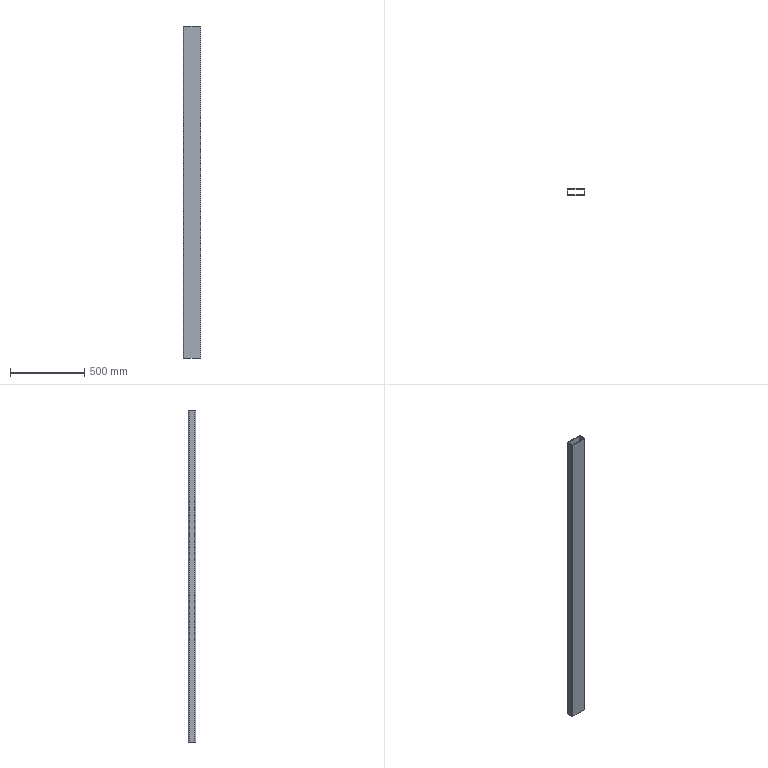Part | SolidWorks | features Extrusion 1, Shell 1 | 1 solid | 18 faces | box 120 x 50 x 2240 mm | volume 2856892 mm3 | plane 10 | cylinder 8 | commonest cylinder face diameters 2 x4 10 x4
STEP:
#1=CARTESIAN_POINT('',(-55.,25.,0.));
#2=VERTEX_POINT('',#1);
#3=CARTESIAN_POINT('',(-60.,20.,0.));
#4=VERTEX_POINT('',#3);
#5=CARTESIAN_POINT('',(-55.,20.,0.));
#6=DIRECTION('',(0.,0.,1.));
#7=DIRECTION('',(1.,0.,0.));
#8=AXIS2_PLACEMENT_3D('',#5,#6,#7);
#9=CIRCLE('',#8,5.);
#10=EDGE_CURVE('',#2,#4,#9,.T.);
#11=ORIENTED_EDGE('',*,*,#10,.T.);
#12=CARTESIAN_POINT('',(-60.,20.,2240.));
#13=VERTEX_POINT('',#12);
#14=CARTESIAN_POINT('',(-60.,20.,2240.));
#15=DIRECTION('',(0.,0.,-1.));
#16=VECTOR('',#15,1000.);
#17=LINE('',#14,#16);
#18=EDGE_CURVE('',#13,#4,#17,.T.);
#19=ORIENTED_EDGE('',*,*,#18,.F.);
#20=CARTESIAN_POINT('',(-55.,25.,2240.));
#21=VERTEX_POINT('',#20);
#22=CARTESIAN_POINT('',(-55.,20.,2240.));
#23=DIRECTION('',(0.,0.,1.));
#24=DIRECTION('',(1.,0.,0.));
#25=AXIS2_PLACEMENT_3D('',#22,#23,#24);
#26=CIRCLE('',#25,5.);
#27=EDGE_CURVE('',#21,#13,#26,.T.);
#28=ORIENTED_EDGE('',*,*,#27,.F.);
#29=CARTESIAN_POINT('',(-55.,25.,2240.));
#30=DIRECTION('',(0.,0.,-1.));
#31=VECTOR('',#30,1000.);
#32=LINE('',#29,#31);
#33=EDGE_CURVE('',#21,#2,#32,.T.);
#34=ORIENTED_EDGE('',*,*,#33,.T.);
#35=EDGE_LOOP('',(#11,#19,#28,#34));
#36=FACE_OUTER_BOUND('',#35,.T.);
#37=CARTESIAN_POINT('',(-55.,20.,2240.));
#38=DIRECTION('',(0.,0.,-1.));
#39=DIRECTION('',(-1.,0.,0.));
#40=AXIS2_PLACEMENT_3D('',#37,#38,#39);
#41=CYLINDRICAL_SURFACE('',#40,5.);
#42=ADVANCED_FACE('',(#36),#41,.T.);
#43=CARTESIAN_POINT('',(-60.,-20.,0.));
#44=VERTEX_POINT('',#43);
#45=CARTESIAN_POINT('',(-60.,20.,0.));
#46=DIRECTION('',(0.,-1.,0.));
#47=VECTOR('',#46,1000.);
#48=LINE('',#45,#47);
#49=EDGE_CURVE('',#4,#44,#48,.T.);
#50=ORIENTED_EDGE('',*,*,#49,.T.);
#51=CARTESIAN_POINT('',(-60.,-20.,2240.));
#52=VERTEX_POINT('',#51);
#53=CARTESIAN_POINT('',(-60.,-20.,2240.));
#54=DIRECTION('',(0.,0.,-1.));
#55=VECTOR('',#54,1000.);
#56=LINE('',#53,#55);
#57=EDGE_CURVE('',#52,#44,#56,.T.);
#58=ORIENTED_EDGE('',*,*,#57,.F.);
#59=CARTESIAN_POINT('',(-60.,20.,2240.));
#60=DIRECTION('',(0.,-1.,0.));
#61=VECTOR('',#60,1000.);
#62=LINE('',#59,#61);
#63=EDGE_CURVE('',#13,#52,#62,.T.);
#64=ORIENTED_EDGE('',*,*,#63,.F.);
#65=ORIENTED_EDGE('',*,*,#18,.T.);
#66=EDGE_LOOP('',(#50,#58,#64,#65));
#67=FACE_OUTER_BOUND('',#66,.T.);
#68=CARTESIAN_POINT('',(-60.,20.,2240.));
#69=DIRECTION('',(1.,0.,0.));
#70=DIRECTION('',(0.,1.,0.));
#71=AXIS2_PLACEMENT_3D('',#68,#69,#70);
#72=PLANE('',#71);
#73=ADVANCED_FACE('',(#67),#72,.F.);
#74=CARTESIAN_POINT('',(-55.,-25.,0.));
#75=VERTEX_POINT('',#74);
#76=CARTESIAN_POINT('',(-55.,-20.,0.));
#77=DIRECTION('',(0.,0.,-1.));
#78=DIRECTION('',(-1.,0.,0.));
#79=AXIS2_PLACEMENT_3D('',#76,#77,#78);
#80=CIRCLE('',#79,5.);
#81=EDGE_CURVE('',#75,#44,#80,.T.);
#82=ORIENTED_EDGE('',*,*,#81,.F.);
#83=CARTESIAN_POINT('',(-55.,-25.,2240.));
#84=VERTEX_POINT('',#83);
#85=CARTESIAN_POINT('',(-55.,-25.,2240.));
#86=DIRECTION('',(0.,0.,-1.));
#87=VECTOR('',#86,1000.);
#88=LINE('',#85,#87);
#89=EDGE_CURVE('',#84,#75,#88,.T.);
#90=ORIENTED_EDGE('',*,*,#89,.F.);
#91=CARTESIAN_POINT('',(-55.,-20.,2240.));
#92=DIRECTION('',(0.,0.,-1.));
#93=DIRECTION('',(-1.,0.,0.));
#94=AXIS2_PLACEMENT_3D('',#91,#92,#93);
#95=CIRCLE('',#94,5.);
#96=EDGE_CURVE('',#84,#52,#95,.T.);
#97=ORIENTED_EDGE('',*,*,#96,.T.);
#98=ORIENTED_EDGE('',*,*,#57,.T.);
#99=EDGE_LOOP('',(#82,#90,#97,#98));
#100=FACE_OUTER_BOUND('',#99,.T.);
#101=CARTESIAN_POINT('',(-55.,-20.,2240.));
#102=DIRECTION('',(0.,0.,-1.));
#103=DIRECTION('',(-1.,0.,0.));
#104=AXIS2_PLACEMENT_3D('',#101,#102,#103);
#105=CYLINDRICAL_SURFACE('',#104,5.);
#106=ADVANCED_FACE('',(#100),#105,.T.);
#107=CARTESIAN_POINT('',(55.,-25.,0.));
#108=VERTEX_POINT('',#107);
#109=CARTESIAN_POINT('',(55.,-25.,0.));
#110=DIRECTION('',(-1.,0.,0.));
#111=VECTOR('',#110,1000.);
#112=LINE('',#109,#111);
#113=EDGE_CURVE('',#108,#75,#112,.T.);
#114=ORIENTED_EDGE('',*,*,#113,.F.);
#115=CARTESIAN_POINT('',(55.,-25.,2240.));
#116=VERTEX_POINT('',#115);
#117=CARTESIAN_POINT('',(55.,-25.,2240.));
#118=DIRECTION('',(0.,0.,-1.));
#119=VECTOR('',#118,1000.);
#120=LINE('',#117,#119);
#121=EDGE_CURVE('',#116,#108,#120,.T.);
#122=ORIENTED_EDGE('',*,*,#121,.F.);
#123=CARTESIAN_POINT('',(55.,-25.,2240.));
#124=DIRECTION('',(-1.,0.,0.));
#125=VECTOR('',#124,1000.);
#126=LINE('',#123,#125);
#127=EDGE_CURVE('',#116,#84,#126,.T.);
#128=ORIENTED_EDGE('',*,*,#127,.T.);
#129=ORIENTED_EDGE('',*,*,#89,.T.);
#130=EDGE_LOOP('',(#114,#122,#128,#129));
#131=FACE_OUTER_BOUND('',#130,.T.);
#132=CARTESIAN_POINT('',(55.,-25.,2240.));
#133=DIRECTION('',(0.,-1.,0.));
#134=DIRECTION('',(1.,0.,0.));
#135=AXIS2_PLACEMENT_3D('',#132,#133,#134);
#136=PLANE('',#135);
#137=ADVANCED_FACE('',(#131),#136,.T.);
#138=CARTESIAN_POINT('',(60.,-20.,0.));
#139=VERTEX_POINT('',#138);
#140=CARTESIAN_POINT('',(55.,-20.,0.));
#141=DIRECTION('',(0.,0.,-1.));
#142=DIRECTION('',(-1.,0.,0.));
#143=AXIS2_PLACEMENT_3D('',#140,#141,#142);
#144=CIRCLE('',#143,5.);
#145=EDGE_CURVE('',#139,#108,#144,.T.);
#146=ORIENTED_EDGE('',*,*,#145,.F.);
#147=CARTESIAN_POINT('',(60.,-20.,2240.));
#148=VERTEX_POINT('',#147);
#149=CARTESIAN_POINT('',(60.,-20.,2240.));
#150=DIRECTION('',(0.,0.,-1.));
#151=VECTOR('',#150,1000.);
#152=LINE('',#149,#151);
#153=EDGE_CURVE('',#148,#139,#152,.T.);
#154=ORIENTED_EDGE('',*,*,#153,.F.);
#155=CARTESIAN_POINT('',(55.,-20.,2240.));
#156=DIRECTION('',(0.,0.,-1.));
#157=DIRECTION('',(-1.,0.,0.));
#158=AXIS2_PLACEMENT_3D('',#155,#156,#157);
#159=CIRCLE('',#158,5.);
#160=EDGE_CURVE('',#148,#116,#159,.T.);
#161=ORIENTED_EDGE('',*,*,#160,.T.);
#162=ORIENTED_EDGE('',*,*,#121,.T.);
#163=EDGE_LOOP('',(#146,#154,#161,#162));
#164=FACE_OUTER_BOUND('',#163,.T.);
#165=CARTESIAN_POINT('',(55.,-20.,2240.));
#166=DIRECTION('',(0.,0.,-1.));
#167=DIRECTION('',(-1.,0.,0.));
#168=AXIS2_PLACEMENT_3D('',#165,#166,#167);
#169=CYLINDRICAL_SURFACE('',#168,5.);
#170=ADVANCED_FACE('',(#164),#169,.T.);
#171=CARTESIAN_POINT('',(60.,20.,0.));
#172=VERTEX_POINT('',#171);
#173=CARTESIAN_POINT('',(60.,20.,0.));
#174=DIRECTION('',(0.,-1.,0.));
#175=VECTOR('',#174,1000.);
#176=LINE('',#173,#175);
#177=EDGE_CURVE('',#172,#139,#176,.T.);
#178=ORIENTED_EDGE('',*,*,#177,.F.);
#179=CARTESIAN_POINT('',(60.,20.,2240.));
#180=VERTEX_POINT('',#179);
#181=CARTESIAN_POINT('',(60.,20.,2240.));
#182=DIRECTION('',(0.,0.,-1.));
#183=VECTOR('',#182,1000.);
#184=LINE('',#181,#183);
#185=EDGE_CURVE('',#180,#172,#184,.T.);
#186=ORIENTED_EDGE('',*,*,#185,.F.);
#187=CARTESIAN_POINT('',(60.,20.,2240.));
#188=DIRECTION('',(0.,-1.,0.));
#189=VECTOR('',#188,1000.);
#190=LINE('',#187,#189);
#191=EDGE_CURVE('',#180,#148,#190,.T.);
#192=ORIENTED_EDGE('',*,*,#191,.T.);
#193=ORIENTED_EDGE('',*,*,#153,.T.);
#194=EDGE_LOOP('',(#178,#186,#192,#193));
#195=FACE_OUTER_BOUND('',#194,.T.);
#196=CARTESIAN_POINT('',(60.,20.,2240.));
#197=DIRECTION('',(1.,0.,0.));
#198=DIRECTION('',(0.,1.,0.));
#199=AXIS2_PLACEMENT_3D('',#196,#197,#198);
#200=PLANE('',#199);
#201=ADVANCED_FACE('',(#195),#200,.T.);
#202=CARTESIAN_POINT('',(55.,25.,0.));
#203=VERTEX_POINT('',#202);
#204=CARTESIAN_POINT('',(55.,20.,0.));
#205=DIRECTION('',(0.,0.,-1.));
#206=DIRECTION('',(-1.,0.,0.));
#207=AXIS2_PLACEMENT_3D('',#204,#205,#206);
#208=CIRCLE('',#207,5.);
#209=EDGE_CURVE('',#203,#172,#208,.T.);
#210=ORIENTED_EDGE('',*,*,#209,.F.);
#211=CARTESIAN_POINT('',(55.,25.,2240.));
#212=VERTEX_POINT('',#211);
#213=CARTESIAN_POINT('',(55.,25.,2240.));
#214=DIRECTION('',(0.,0.,-1.));
#215=VECTOR('',#214,1000.);
#216=LINE('',#213,#215);
#217=EDGE_CURVE('',#212,#203,#216,.T.);
#218=ORIENTED_EDGE('',*,*,#217,.F.);
#219=CARTESIAN_POINT('',(55.,20.,2240.));
#220=DIRECTION('',(0.,0.,-1.));
#221=DIRECTION('',(-1.,0.,0.));
#222=AXIS2_PLACEMENT_3D('',#219,#220,#221);
#223=CIRCLE('',#222,5.);
#224=EDGE_CURVE('',#212,#180,#223,.T.);
#225=ORIENTED_EDGE('',*,*,#224,.T.);
#226=ORIENTED_EDGE('',*,*,#185,.T.);
#227=EDGE_LOOP('',(#210,#218,#225,#226));
#228=FACE_OUTER_BOUND('',#227,.T.);
#229=CARTESIAN_POINT('',(55.,20.,2240.));
#230=DIRECTION('',(0.,0.,-1.));
#231=DIRECTION('',(-1.,0.,0.));
#232=AXIS2_PLACEMENT_3D('',#229,#230,#231);
#233=CYLINDRICAL_SURFACE('',#232,5.);
#234=ADVANCED_FACE('',(#228),#233,.T.);
#235=CARTESIAN_POINT('',(55.,25.,0.));
#236=DIRECTION('',(-1.,0.,0.));
#237=VECTOR('',#236,1000.);
#238=LINE('',#235,#237);
#239=EDGE_CURVE('',#203,#2,#238,.T.);
#240=ORIENTED_EDGE('',*,*,#239,.T.);
#241=ORIENTED_EDGE('',*,*,#33,.F.);
#242=CARTESIAN_POINT('',(55.,25.,2240.));
#243=DIRECTION('',(-1.,0.,0.));
#244=VECTOR('',#243,1000.);
#245=LINE('',#242,#244);
#246=EDGE_CURVE('',#212,#21,#245,.T.);
#247=ORIENTED_EDGE('',*,*,#246,.F.);
#248=ORIENTED_EDGE('',*,*,#217,.T.);
#249=EDGE_LOOP('',(#240,#241,#247,#248));
#250=FACE_OUTER_BOUND('',#249,.T.);
#251=CARTESIAN_POINT('',(55.,25.,2240.));
#252=DIRECTION('',(0.,-1.,0.));
#253=DIRECTION('',(1.,0.,0.));
#254=AXIS2_PLACEMENT_3D('',#251,#252,#253);
#255=PLANE('',#254);
#256=ADVANCED_FACE('',(#250),#255,.F.);
#257=CARTESIAN_POINT('',(-55.,21.,2240.));
#258=VERTEX_POINT('',#257);
#259=CARTESIAN_POINT('',(-56.,20.,2240.));
#260=VERTEX_POINT('',#259);
#261=CARTESIAN_POINT('',(-55.,20.,2240.));
#262=DIRECTION('',(0.,0.,1.));
#263=DIRECTION('',(1.,0.,0.));
#264=AXIS2_PLACEMENT_3D('',#261,#262,#263);
#265=CIRCLE('',#264,1.);
#266=EDGE_CURVE('',#258,#260,#265,.T.);
#267=ORIENTED_EDGE('',*,*,#266,.F.);
#268=CARTESIAN_POINT('',(55.,21.,2240.));
#269=VERTEX_POINT('',#268);
#270=CARTESIAN_POINT('',(55.,21.,2240.));
#271=DIRECTION('',(-1.,0.,0.));
#272=VECTOR('',#271,1000.);
#273=LINE('',#270,#272);
#274=EDGE_CURVE('',#269,#258,#273,.T.);
#275=ORIENTED_EDGE('',*,*,#274,.F.);
#276=CARTESIAN_POINT('',(56.,20.,2240.));
#277=VERTEX_POINT('',#276);
#278=CARTESIAN_POINT('',(55.,20.,2240.));
#279=DIRECTION('',(0.,0.,-1.));
#280=DIRECTION('',(1.,0.,0.));
#281=AXIS2_PLACEMENT_3D('',#278,#279,#280);
#282=CIRCLE('',#281,1.);
#283=EDGE_CURVE('',#269,#277,#282,.T.);
#284=ORIENTED_EDGE('',*,*,#283,.T.);
#285=CARTESIAN_POINT('',(56.,-20.,2240.));
#286=VERTEX_POINT('',#285);
#287=CARTESIAN_POINT('',(56.,20.,2240.));
#288=DIRECTION('',(0.,-1.,0.));
#289=VECTOR('',#288,1000.);
#290=LINE('',#287,#289);
#291=EDGE_CURVE('',#277,#286,#290,.T.);
#292=ORIENTED_EDGE('',*,*,#291,.T.);
#293=CARTESIAN_POINT('',(55.,-21.,2240.));
#294=VERTEX_POINT('',#293);
#295=CARTESIAN_POINT('',(55.,-20.,2240.));
#296=DIRECTION('',(0.,0.,-1.));
#297=DIRECTION('',(1.,0.,0.));
#298=AXIS2_PLACEMENT_3D('',#295,#296,#297);
#299=CIRCLE('',#298,1.);
#300=EDGE_CURVE('',#286,#294,#299,.T.);
#301=ORIENTED_EDGE('',*,*,#300,.T.);
#302=CARTESIAN_POINT('',(-55.,-21.,2240.));
#303=VERTEX_POINT('',#302);
#304=CARTESIAN_POINT('',(55.,-21.,2240.));
#305=DIRECTION('',(-1.,0.,0.));
#306=VECTOR('',#305,1000.);
#307=LINE('',#304,#306);
#308=EDGE_CURVE('',#294,#303,#307,.T.);
#309=ORIENTED_EDGE('',*,*,#308,.T.);
#310=CARTESIAN_POINT('',(-56.,-20.,2240.));
#311=VERTEX_POINT('',#310);
#312=CARTESIAN_POINT('',(-55.,-20.,2240.));
#313=DIRECTION('',(0.,0.,-1.));
#314=DIRECTION('',(1.,0.,0.));
#315=AXIS2_PLACEMENT_3D('',#312,#313,#314);
#316=CIRCLE('',#315,1.);
#317=EDGE_CURVE('',#303,#311,#316,.T.);
#318=ORIENTED_EDGE('',*,*,#317,.T.);
#319=CARTESIAN_POINT('',(-56.,20.,2240.));
#320=DIRECTION('',(0.,-1.,0.));
#321=VECTOR('',#320,1000.);
#322=LINE('',#319,#321);
#323=EDGE_CURVE('',#260,#311,#322,.T.);
#324=ORIENTED_EDGE('',*,*,#323,.F.);
#325=EDGE_LOOP('',(#267,#275,#284,#292,#301,#309,#318,#324));
#326=FACE_BOUND('',#325,.T.);
#327=ORIENTED_EDGE('',*,*,#27,.T.);
#328=ORIENTED_EDGE('',*,*,#63,.T.);
#329=ORIENTED_EDGE('',*,*,#96,.F.);
#330=ORIENTED_EDGE('',*,*,#127,.F.);
#331=ORIENTED_EDGE('',*,*,#160,.F.);
#332=ORIENTED_EDGE('',*,*,#191,.F.);
#333=ORIENTED_EDGE('',*,*,#224,.F.);
#334=ORIENTED_EDGE('',*,*,#246,.T.);
#335=EDGE_LOOP('',(#327,#328,#329,#330,#331,#332,#333,#334));
#336=FACE_OUTER_BOUND('',#335,.T.);
#337=CARTESIAN_POINT('',(-55.,20.,2240.));
#338=DIRECTION('',(0.,0.,1.));
#339=DIRECTION('',(1.,0.,0.));
#340=AXIS2_PLACEMENT_3D('',#337,#338,#339);
#341=PLANE('',#340);
#342=ADVANCED_FACE('',(#326,#336),#341,.T.);
#343=CARTESIAN_POINT('',(55.,21.,0.));
#344=VERTEX_POINT('',#343);
#345=CARTESIAN_POINT('',(-55.,21.,0.));
#346=VERTEX_POINT('',#345);
#347=CARTESIAN_POINT('',(55.,21.,0.));
#348=DIRECTION('',(-1.,0.,0.));
#349=VECTOR('',#348,1000.);
#350=LINE('',#347,#349);
#351=EDGE_CURVE('',#344,#346,#350,.T.);
#352=ORIENTED_EDGE('',*,*,#351,.T.);
#353=CARTESIAN_POINT('',(-56.,20.,0.));
#354=VERTEX_POINT('',#353);
#355=CARTESIAN_POINT('',(-55.,20.,0.));
#356=DIRECTION('',(0.,0.,1.));
#357=DIRECTION('',(1.,0.,0.));
#358=AXIS2_PLACEMENT_3D('',#355,#356,#357);
#359=CIRCLE('',#358,1.);
#360=EDGE_CURVE('',#346,#354,#359,.T.);
#361=ORIENTED_EDGE('',*,*,#360,.T.);
#362=CARTESIAN_POINT('',(-56.,-20.,0.));
#363=VERTEX_POINT('',#362);
#364=CARTESIAN_POINT('',(-56.,20.,0.));
#365=DIRECTION('',(0.,-1.,0.));
#366=VECTOR('',#365,1000.);
#367=LINE('',#364,#366);
#368=EDGE_CURVE('',#354,#363,#367,.T.);
#369=ORIENTED_EDGE('',*,*,#368,.T.);
#370=CARTESIAN_POINT('',(-55.,-21.,0.));
#371=VERTEX_POINT('',#370);
#372=CARTESIAN_POINT('',(-55.,-20.,0.));
#373=DIRECTION('',(0.,0.,-1.));
#374=DIRECTION('',(1.,0.,0.));
#375=AXIS2_PLACEMENT_3D('',#372,#373,#374);
#376=CIRCLE('',#375,1.);
#377=EDGE_CURVE('',#371,#363,#376,.T.);
#378=ORIENTED_EDGE('',*,*,#377,.F.);
#379=CARTESIAN_POINT('',(55.,-21.,0.));
#380=VERTEX_POINT('',#379);
#381=CARTESIAN_POINT('',(55.,-21.,0.));
#382=DIRECTION('',(-1.,0.,0.));
#383=VECTOR('',#382,1000.);
#384=LINE('',#381,#383);
#385=EDGE_CURVE('',#380,#371,#384,.T.);
#386=ORIENTED_EDGE('',*,*,#385,.F.);
#387=CARTESIAN_POINT('',(56.,-20.,0.));
#388=VERTEX_POINT('',#387);
#389=CARTESIAN_POINT('',(55.,-20.,0.));
#390=DIRECTION('',(0.,0.,-1.));
#391=DIRECTION('',(1.,0.,0.));
#392=AXIS2_PLACEMENT_3D('',#389,#390,#391);
#393=CIRCLE('',#392,1.);
#394=EDGE_CURVE('',#388,#380,#393,.T.);
#395=ORIENTED_EDGE('',*,*,#394,.F.);
#396=CARTESIAN_POINT('',(56.,20.,0.));
#397=VERTEX_POINT('',#396);
#398=CARTESIAN_POINT('',(56.,20.,0.));
#399=DIRECTION('',(0.,-1.,0.));
#400=VECTOR('',#399,1000.);
#401=LINE('',#398,#400);
#402=EDGE_CURVE('',#397,#388,#401,.T.);
#403=ORIENTED_EDGE('',*,*,#402,.F.);
#404=CARTESIAN_POINT('',(55.,20.,0.));
#405=DIRECTION('',(0.,0.,-1.));
#406=DIRECTION('',(1.,0.,0.));
#407=AXIS2_PLACEMENT_3D('',#404,#405,#406);
#408=CIRCLE('',#407,1.);
#409=EDGE_CURVE('',#344,#397,#408,.T.);
#410=ORIENTED_EDGE('',*,*,#409,.F.);
#411=EDGE_LOOP('',(#352,#361,#369,#378,#386,#395,#403,#410));
#412=FACE_BOUND('',#411,.T.);
#413=ORIENTED_EDGE('',*,*,#10,.F.);
#414=ORIENTED_EDGE('',*,*,#239,.F.);
#415=ORIENTED_EDGE('',*,*,#209,.T.);
#416=ORIENTED_EDGE('',*,*,#177,.T.);
#417=ORIENTED_EDGE('',*,*,#145,.T.);
#418=ORIENTED_EDGE('',*,*,#113,.T.);
#419=ORIENTED_EDGE('',*,*,#81,.T.);
#420=ORIENTED_EDGE('',*,*,#49,.F.);
#421=EDGE_LOOP('',(#413,#414,#415,#416,#417,#418,#419,#420));
#422=FACE_OUTER_BOUND('',#421,.T.);
#423=CARTESIAN_POINT('',(-55.,20.,0.));
#424=DIRECTION('',(0.,0.,1.));
#425=DIRECTION('',(1.,0.,0.));
#426=AXIS2_PLACEMENT_3D('',#423,#424,#425);
#427=PLANE('',#426);
#428=ADVANCED_FACE('',(#412,#422),#427,.F.);
#429=ORIENTED_EDGE('',*,*,#360,.F.);
#430=CARTESIAN_POINT('',(-55.,21.,2240.));
#431=DIRECTION('',(0.,0.,-1.));
#432=VECTOR('',#431,1000.);
#433=LINE('',#430,#432);
#434=EDGE_CURVE('',#258,#346,#433,.T.);
#435=ORIENTED_EDGE('',*,*,#434,.F.);
#436=ORIENTED_EDGE('',*,*,#266,.T.);
#437=CARTESIAN_POINT('',(-56.,20.,2240.));
#438=DIRECTION('',(0.,0.,-1.));
#439=VECTOR('',#438,1000.);
#440=LINE('',#437,#439);
#441=EDGE_CURVE('',#260,#354,#440,.T.);
#442=ORIENTED_EDGE('',*,*,#441,.T.);
#443=EDGE_LOOP('',(#429,#435,#436,#442));
#444=FACE_OUTER_BOUND('',#443,.T.);
#445=CARTESIAN_POINT('',(-55.,20.,2240.));
#446=DIRECTION('',(0.,0.,-1.));
#447=DIRECTION('',(-1.,0.,0.));
#448=AXIS2_PLACEMENT_3D('',#445,#446,#447);
#449=CYLINDRICAL_SURFACE('',#448,1.);
#450=ADVANCED_FACE('',(#444),#449,.F.);
#451=ORIENTED_EDGE('',*,*,#368,.F.);
#452=ORIENTED_EDGE('',*,*,#441,.F.);
#453=ORIENTED_EDGE('',*,*,#323,.T.);
#454=CARTESIAN_POINT('',(-56.,-20.,2240.));
#455=DIRECTION('',(0.,0.,-1.));
#456=VECTOR('',#455,1000.);
#457=LINE('',#454,#456);
#458=EDGE_CURVE('',#311,#363,#457,.T.);
#459=ORIENTED_EDGE('',*,*,#458,.T.);
#460=EDGE_LOOP('',(#451,#452,#453,#459));
#461=FACE_OUTER_BOUND('',#460,.T.);
#462=CARTESIAN_POINT('',(-56.,20.,2240.));
#463=DIRECTION('',(1.,0.,0.));
#464=DIRECTION('',(0.,1.,0.));
#465=AXIS2_PLACEMENT_3D('',#462,#463,#464);
#466=PLANE('',#465);
#467=ADVANCED_FACE('',(#461),#466,.T.);
#468=ORIENTED_EDGE('',*,*,#377,.T.);
#469=ORIENTED_EDGE('',*,*,#458,.F.);
#470=ORIENTED_EDGE('',*,*,#317,.F.);
#471=CARTESIAN_POINT('',(-55.,-21.,2240.));
#472=DIRECTION('',(0.,0.,-1.));
#473=VECTOR('',#472,1000.);
#474=LINE('',#471,#473);
#475=EDGE_CURVE('',#303,#371,#474,.T.);
#476=ORIENTED_EDGE('',*,*,#475,.T.);
#477=EDGE_LOOP('',(#468,#469,#470,#476));
#478=FACE_OUTER_BOUND('',#477,.T.);
#479=CARTESIAN_POINT('',(-55.,-20.,2240.));
#480=DIRECTION('',(0.,0.,-1.));
#481=DIRECTION('',(-1.,0.,0.));
#482=AXIS2_PLACEMENT_3D('',#479,#480,#481);
#483=CYLINDRICAL_SURFACE('',#482,1.);
#484=ADVANCED_FACE('',(#478),#483,.F.);
#485=ORIENTED_EDGE('',*,*,#385,.T.);
#486=ORIENTED_EDGE('',*,*,#475,.F.);
#487=ORIENTED_EDGE('',*,*,#308,.F.);
#488=CARTESIAN_POINT('',(55.,-21.,2240.));
#489=DIRECTION('',(0.,0.,-1.));
#490=VECTOR('',#489,1000.);
#491=LINE('',#488,#490);
#492=EDGE_CURVE('',#294,#380,#491,.T.);
#493=ORIENTED_EDGE('',*,*,#492,.T.);
#494=EDGE_LOOP('',(#485,#486,#487,#493));
#495=FACE_OUTER_BOUND('',#494,.T.);
#496=CARTESIAN_POINT('',(55.,-21.,2240.));
#497=DIRECTION('',(0.,-1.,0.));
#498=DIRECTION('',(1.,0.,0.));
#499=AXIS2_PLACEMENT_3D('',#496,#497,#498);
#500=PLANE('',#499);
#501=ADVANCED_FACE('',(#495),#500,.F.);
#502=ORIENTED_EDGE('',*,*,#394,.T.);
#503=ORIENTED_EDGE('',*,*,#492,.F.);
#504=ORIENTED_EDGE('',*,*,#300,.F.);
#505=CARTESIAN_POINT('',(56.,-20.,2240.));
#506=DIRECTION('',(0.,0.,-1.));
#507=VECTOR('',#506,1000.);
#508=LINE('',#505,#507);
#509=EDGE_CURVE('',#286,#388,#508,.T.);
#510=ORIENTED_EDGE('',*,*,#509,.T.);
#511=EDGE_LOOP('',(#502,#503,#504,#510));
#512=FACE_OUTER_BOUND('',#511,.T.);
#513=CARTESIAN_POINT('',(55.,-20.,2240.));
#514=DIRECTION('',(0.,0.,-1.));
#515=DIRECTION('',(-1.,0.,0.));
#516=AXIS2_PLACEMENT_3D('',#513,#514,#515);
#517=CYLINDRICAL_SURFACE('',#516,1.);
#518=ADVANCED_FACE('',(#512),#517,.F.);
#519=ORIENTED_EDGE('',*,*,#402,.T.);
#520=ORIENTED_EDGE('',*,*,#509,.F.);
#521=ORIENTED_EDGE('',*,*,#291,.F.);
#522=CARTESIAN_POINT('',(56.,20.,2240.));
#523=DIRECTION('',(0.,0.,-1.));
#524=VECTOR('',#523,1000.);
#525=LINE('',#522,#524);
#526=EDGE_CURVE('',#277,#397,#525,.T.);
#527=ORIENTED_EDGE('',*,*,#526,.T.);
#528=EDGE_LOOP('',(#519,#520,#521,#527));
#529=FACE_OUTER_BOUND('',#528,.T.);
#530=CARTESIAN_POINT('',(56.,20.,2240.));
#531=DIRECTION('',(1.,0.,0.));
#532=DIRECTION('',(0.,1.,0.));
#533=AXIS2_PLACEMENT_3D('',#530,#531,#532);
#534=PLANE('',#533);
#535=ADVANCED_FACE('',(#529),#534,.F.);
#536=ORIENTED_EDGE('',*,*,#409,.T.);
#537=ORIENTED_EDGE('',*,*,#526,.F.);
#538=ORIENTED_EDGE('',*,*,#283,.F.);
#539=CARTESIAN_POINT('',(55.,21.,2240.));
#540=DIRECTION('',(0.,0.,-1.));
#541=VECTOR('',#540,1000.);
#542=LINE('',#539,#541);
#543=EDGE_CURVE('',#269,#344,#542,.T.);
#544=ORIENTED_EDGE('',*,*,#543,.T.);
#545=EDGE_LOOP('',(#536,#537,#538,#544));
#546=FACE_OUTER_BOUND('',#545,.T.);
#547=CARTESIAN_POINT('',(55.,20.,2240.));
#548=DIRECTION('',(0.,0.,-1.));
#549=DIRECTION('',(-1.,0.,0.));
#550=AXIS2_PLACEMENT_3D('',#547,#548,#549);
#551=CYLINDRICAL_SURFACE('',#550,1.);
#552=ADVANCED_FACE('',(#546),#551,.F.);
#553=ORIENTED_EDGE('',*,*,#351,.F.);
#554=ORIENTED_EDGE('',*,*,#543,.F.);
#555=ORIENTED_EDGE('',*,*,#274,.T.);
#556=ORIENTED_EDGE('',*,*,#434,.T.);
#557=EDGE_LOOP('',(#553,#554,#555,#556));
#558=FACE_OUTER_BOUND('',#557,.T.);
#559=CARTESIAN_POINT('',(55.,21.,2240.));
#560=DIRECTION('',(0.,-1.,0.));
#561=DIRECTION('',(1.,0.,0.));
#562=AXIS2_PLACEMENT_3D('',#559,#560,#561);
#563=PLANE('',#562);
#564=ADVANCED_FACE('',(#558),#563,.T.);
#565=CLOSED_SHELL('',(#42,#73,#106,#137,#170,#201,#234,#256,#342,#428,#450,#467,#484,#501,#518,#535,#552,#564));
#566=MANIFOLD_SOLID_BREP('',#565);
#567=CARTESIAN_POINT('',(0.,0.,0.));
#568=DIRECTION('',(0.,0.,1.));
#569=DIRECTION('',(1.,0.,0.));
#570=AXIS2_PLACEMENT_3D('',#567,#568,#569);
#571=(LENGTH_UNIT()NAMED_UNIT(*)SI_UNIT(.MILLI.,.METRE.));
#572=UNCERTAINTY_MEASURE_WITH_UNIT(LENGTH_MEASURE(0.00001),#571,'','');
#573=(NAMED_UNIT(*)PLANE_ANGLE_UNIT()SI_UNIT($,.RADIAN.));
#574=(NAMED_UNIT(*)SI_UNIT($,.STERADIAN.)SOLID_ANGLE_UNIT());
#575=(GEOMETRIC_REPRESENTATION_CONTEXT(3)GLOBAL_UNCERTAINTY_ASSIGNED_CONTEXT((#572))GLOBAL_UNIT_ASSIGNED_CONTEXT((#571,#573,#574))REPRESENTATION_CONTEXT('',''));
#576=ADVANCED_BREP_SHAPE_REPRESENTATION('',(#566,#570),#575);